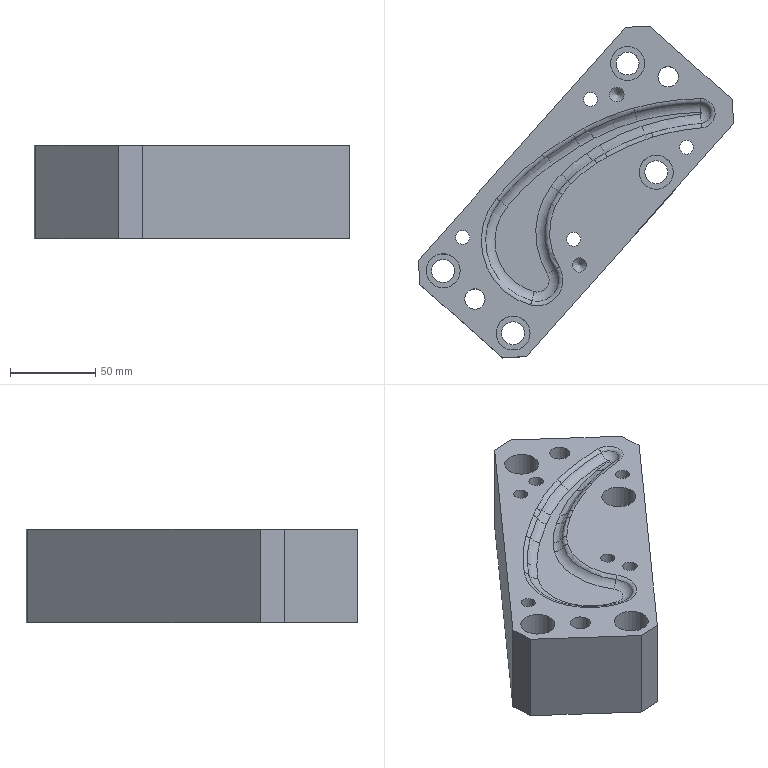Part | NX | features 23 2 | 1 solid | 69 faces | box 185.139 x 194.875 x 55 mm | volume 840325 mm3 | cylinder 20 | plane 19 | torus 16 | spline 12 | cone 2 | commonest cylinder face diameters 8.2 x4 10.31 x4 13.5 x4 20 x4 8.5 x2 12.001 x2